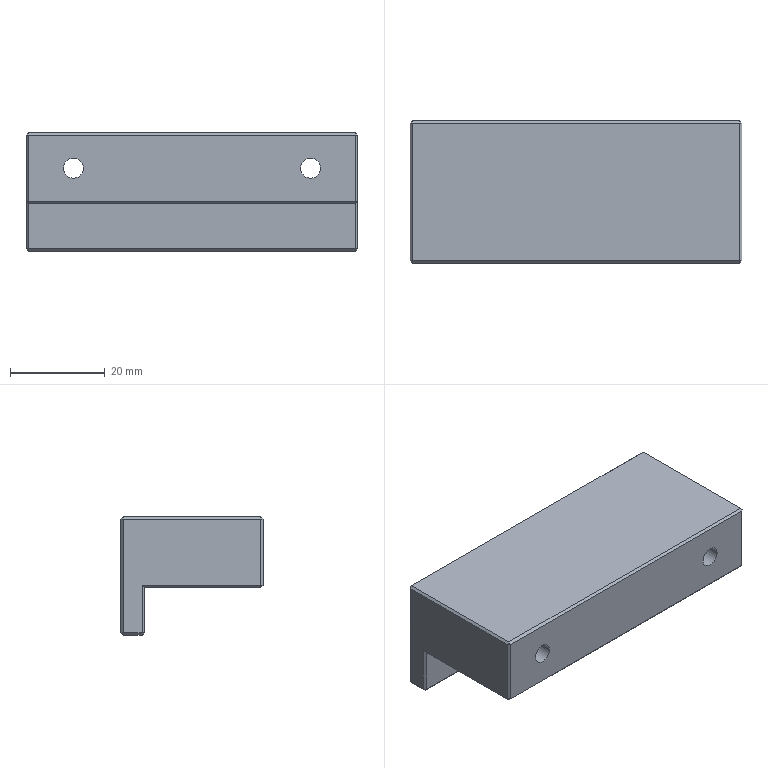Part | STEP file | 06-15 Slide guide block 1 | 1 solid | 45 faces | box 70 x 30 x 25 mm | volume 33661 mm3 | plane 37 | cylinder 8 | commonest cylinder face diameters 4.2 x4 8 x4